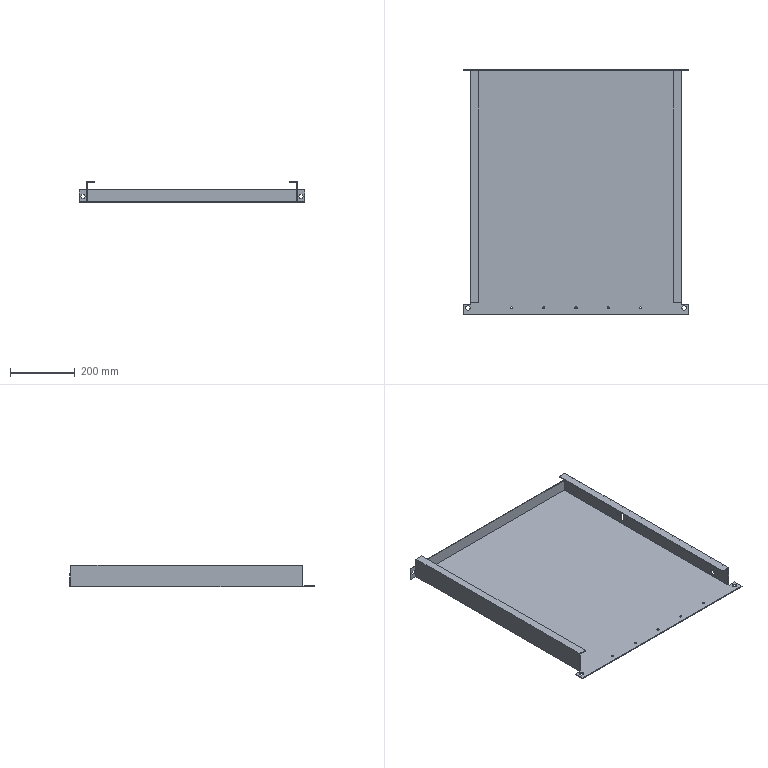Part | SolidWorks | features BaseBody 1 | 1 solid | 66 faces | box 698 x 756 x 66.5 mm | volume 1924391 mm3 | plane 42 | cylinder 24 | commonest cylinder face diameters 6.5 x10 5.5 x8 14 x4 15 x2